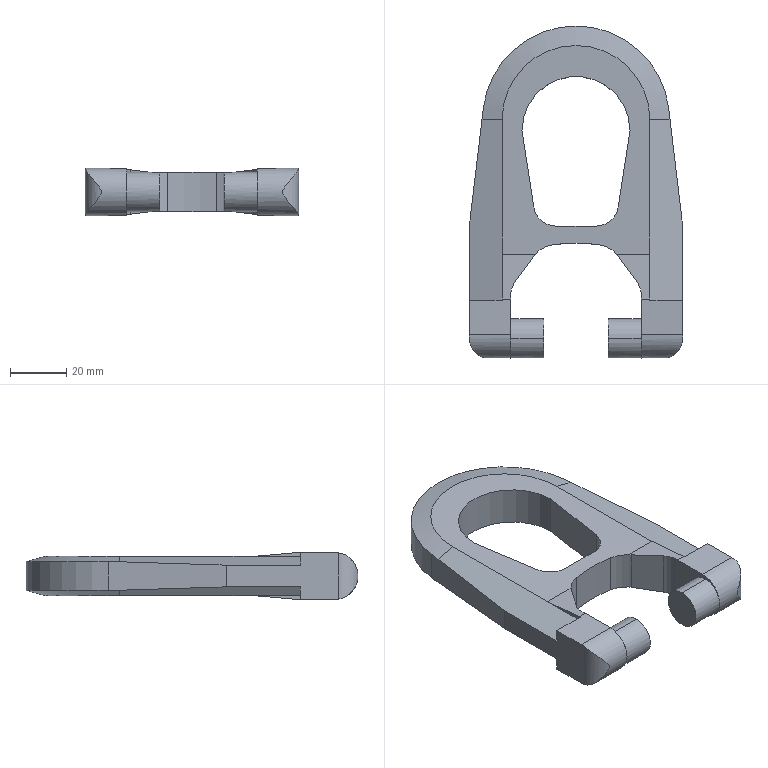Part | STEP file | Support bracket - DSR-C | 1 solid | 54 faces | box 76 x 118.25 x 16.8 mm | volume 64221 mm3 | plane 35 | cylinder 17 | cone 2 | commonest cylinder face diameters 14 x8 16 x2 16.8 x2 20 x2 38.5 x1 66.5 x1